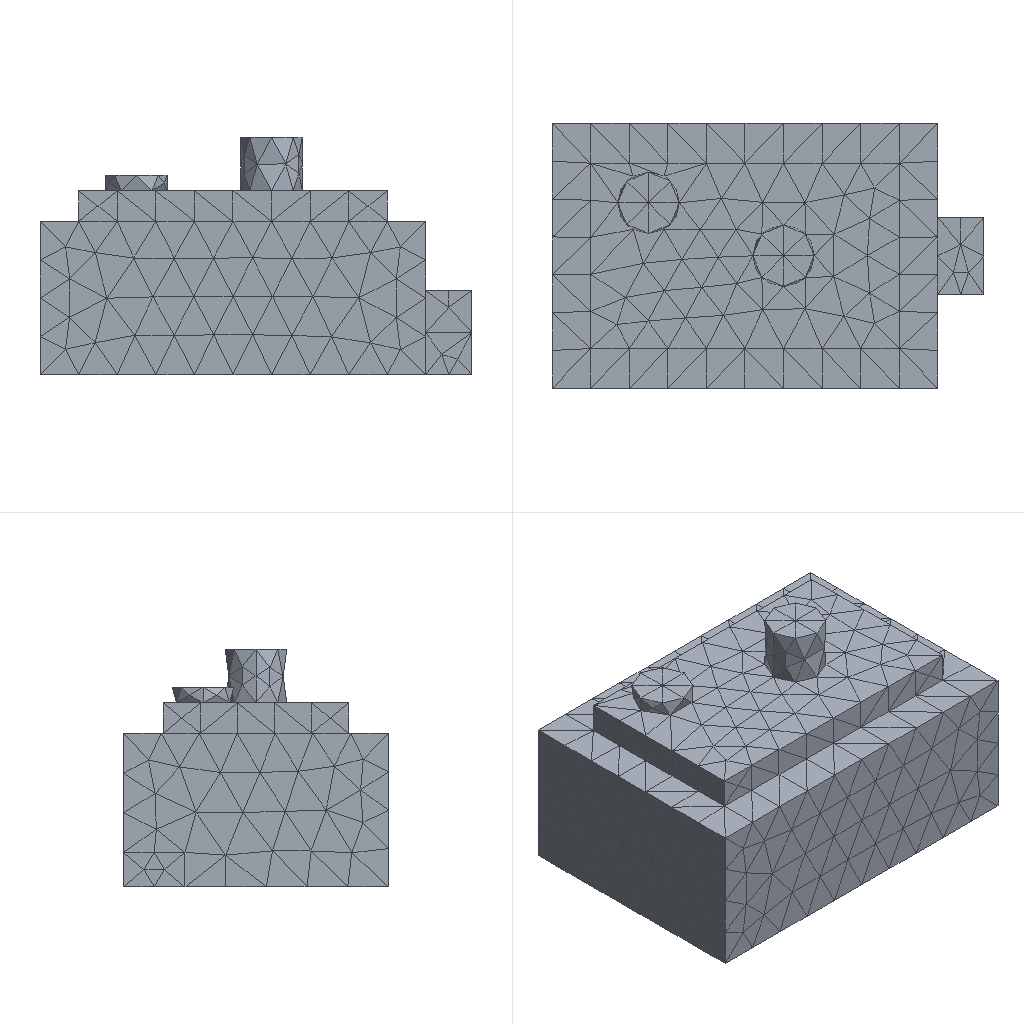Simulation study | ansys mapdl
Set-up summary:
category,name,step,type,value,unit,region
solver,ansys_mapdl
units,mm-N-s-tonne (MPa),,inferred,E=210000 density=
analysis,model,,static
mesh,nodes,,,4537
mesh,elements,,,2720
element_type,SOLID187,,,2720
material,mat 1,,E,210000
material,mat 1,,nu,0.3
load,,model,body load temp,,,all
load,,model,force,"1000 [dir=(0, 0, -1) n=173]",,node list
bc,,model,fixed,"[dofs=UX,UY,UZ n=4797]",,node list
Ansys APDL input file, long lists of numbers shortened:
/COM,ANSYS RELEASE 2026 R1           BUILD 26.1      UP20260202       09:04:29
/PREP7
/NOPR
/TITLE,2
ANTYPE, 0
*IF,_CDRDOFF,EQ,1,THEN     !if solid model was read in
_CDRDOFF=             !reset flag, numoffs already performed
*ELSE              !offset database for the following FE model
NUMOFF,NODE,     4537
NUMOFF,ELEM,     2720
NUMOFF,MAT ,        1
NUMOFF,TYPE,        1
*ENDIF
*SET,_RETURN ,  0.
*SET,_STATUS ,  0.
*SET,_UIQR   ,  173.
*SET,__FLOATPARAMETER__,  4537.
DOF,DELETE
ETBLOCK,        1,        1
(2i9,19a9)
        1      187        0        0        0        0        0        0        0        0        0        0        0        0        0        0        0        0        0        0        0
       -1
NBLOCK,6,SOLID,      4537,      4537
(3i9,6e21.13e3)
        1        0        0-3.4250000000000E+001 3.4500000000000E+001 9.0000000000000E+000
! (4536 more lines like these left out)
N,UNBL,LOC,       -1,
EBLOCK,19,SOLID,      2720,      2720
(19i10)
         1         1         1         1         0         0         0         0        10         0         1      1715      1716      1571      1173      1980      1981      1982      1983
! (5439 more lines like these left out)
        -1
MPTEMP,UNBL, 1, 1,  0.    ,
MPDATA,UNBL, 1,EX  ,       1, 1,  210000.000    ,
MPTEMP,UNBL, 1, 1,  0.    ,
MPDATA,UNBL, 1,NUXY,       1, 1, 0.3    ,
MPTEMP,UNBL, 1, 1,  0.    ,
MPDATA,UNBL, 1,PRXY,       1, 1, 0.3    ,
EXTOPT,ATTR,      0,      0,      0
EXTOPT,ESIZE,  0,  0.
EXTOPT,ACLEAR,      0
TREF,  0.
IRLF,  0
BFUNIF,TEMP,_TINY
ACEL,  0.    ,  0.    ,  0.
OMEGA,  0.    ,  0.    ,  0.
DOMEGA,  0.    ,  0.    ,  0.
CGLOC,  0.    ,  0.    ,  0.
CGOMEGA,  0.    ,  0.    ,  0.
DCGOMG,  0.    ,  0.    ,  0.
KUSE,     0
TIME,  0.
ALPHAD,  0.
BETAD,  0.
DMPRAT,  0.
DMPSTR,  0.
CRPLIM, 0.1    ,   0
CRPLIM,  0.    ,   1
NCNV,     0, 1.000000000E+12,     0,  0.    ,  0.
NEQIT,     0
ERESX,DEFA
DBLOCK,      4797
(i9,a6,2(pg16.9))
        1  UX    0.00000000      0.00000000
! (4796 more lines like these left out)
       -1
FBLOCK,       173
(i9,a6,2(pg16.9))
      823  FZ   -5.78034682      0.00000000
! (172 more lines like these left out)
       -1
/GO
FINISH
Results summary:
result,analysis_type_db,,,static,unstated
result,n_sets,,,1,unstated
result,load_steps[0].set,load_step=1,,1,unstated
result,load_steps[0].substep,load_step=1,,1,unstated
result,load_steps[0].time,load_step=1,,1,unstated
result,load_steps[0].freq,load_step=1,,1,unstated
result,load_steps[0].max_usum,load_step=1,,0.0003752,unstated
result,load_steps[0].max_seqv,load_step=1,,4.373,unstated
result,load_steps[0].reaction_sum.FX,load_step=1,,-1.38023e-11,unstated
result,load_steps[0].reaction_sum.FY,load_step=1,,7.5584e-13,unstated
result,load_steps[0].reaction_sum.FZ,load_step=1,,1000,unstated
result,load_steps[0].reaction_sum.MX,load_step=1,,0,unstated
result,load_steps[0].reaction_sum.MY,load_step=1,,0,unstated
result,load_steps[0].reaction_sum.MZ,load_step=1,,0,unstated
result,convergence,,,results present for all listed sets,unstated